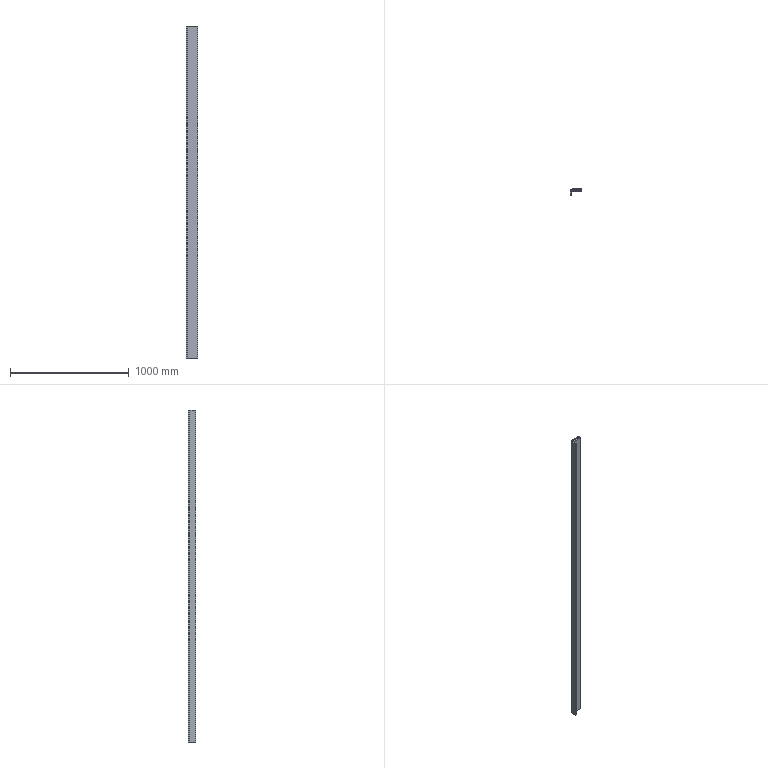Part | SolidWorks | features ICE 3, Extrusion 1, LPattern 1, MirrorPattern 1 | 1 solid | 116 faces | box 100 x 62 x 2800 mm | volume 7257541 mm3 | plane 116